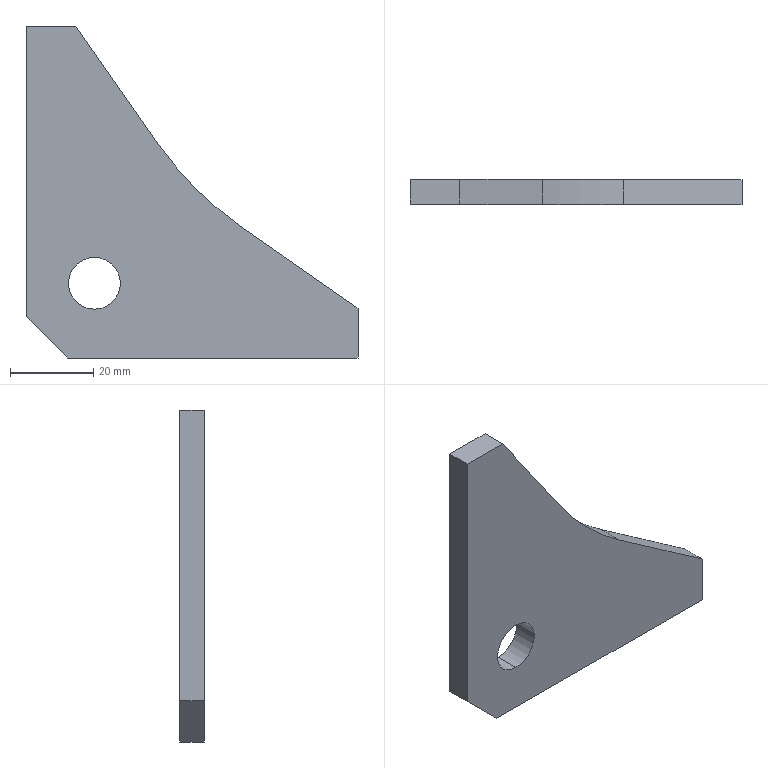Part | SolidWorks | features FlatPattern 1, SMBaseFlange 1, SheetMetal 1 | 1 solid | 12 faces | box 80 x 6 x 80 mm | volume 21113 mm3 | plane 9 | cylinder 3 | commonest cylinder face diameters 12.5 x2 160 x1
STEP:
#1=CARTESIAN_POINT('',(16.5,6.,11.75));
#2=VERTEX_POINT('',#1);
#3=CARTESIAN_POINT('',(16.5,6.,24.25));
#4=VERTEX_POINT('',#3);
#5=CARTESIAN_POINT('',(16.5,6.,18.));
#6=DIRECTION('',(0.,1.,0.));
#7=DIRECTION('',(0.,0.,1.));
#8=AXIS2_PLACEMENT_3D('',#5,#6,#7);
#9=CIRCLE('',#8,6.25);
#10=EDGE_CURVE('',#2,#4,#9,.T.);
#11=ORIENTED_EDGE('',*,*,#10,.T.);
#12=CARTESIAN_POINT('',(16.5,0.,24.25));
#13=VERTEX_POINT('',#12);
#14=CARTESIAN_POINT('',(16.5,6.,24.25));
#15=DIRECTION('',(0.,-1.,0.));
#16=VECTOR('',#15,1000.);
#17=LINE('',#14,#16);
#18=EDGE_CURVE('',#4,#13,#17,.T.);
#19=ORIENTED_EDGE('',*,*,#18,.T.);
#20=CARTESIAN_POINT('',(16.5,0.,11.75));
#21=VERTEX_POINT('',#20);
#22=CARTESIAN_POINT('',(16.5,0.,18.));
#23=DIRECTION('',(0.,1.,0.));
#24=DIRECTION('',(0.,0.,1.));
#25=AXIS2_PLACEMENT_3D('',#22,#23,#24);
#26=CIRCLE('',#25,6.25);
#27=EDGE_CURVE('',#21,#13,#26,.T.);
#28=ORIENTED_EDGE('',*,*,#27,.F.);
#29=CARTESIAN_POINT('',(16.5,6.,11.75));
#30=DIRECTION('',(0.,-1.,0.));
#31=VECTOR('',#30,1000.);
#32=LINE('',#29,#31);
#33=EDGE_CURVE('',#2,#21,#32,.T.);
#34=ORIENTED_EDGE('',*,*,#33,.F.);
#35=EDGE_LOOP('',(#11,#19,#28,#34));
#36=FACE_OUTER_BOUND('',#35,.T.);
#37=CARTESIAN_POINT('',(16.5,6.,18.));
#38=DIRECTION('',(0.,-1.,0.));
#39=DIRECTION('',(0.,0.,-1.));
#40=AXIS2_PLACEMENT_3D('',#37,#38,#39);
#41=CYLINDRICAL_SURFACE('',#40,6.25);
#42=ADVANCED_FACE('',(#36),#41,.F.);
#43=CARTESIAN_POINT('',(80.,6.,12.));
#44=VERTEX_POINT('',#43);
#45=CARTESIAN_POINT('',(80.,6.,0.));
#46=VERTEX_POINT('',#45);
#47=CARTESIAN_POINT('',(80.,6.,12.));
#48=DIRECTION('',(0.,0.,-1.));
#49=VECTOR('',#48,1000.);
#50=LINE('',#47,#49);
#51=EDGE_CURVE('',#44,#46,#50,.T.);
#52=ORIENTED_EDGE('',*,*,#51,.T.);
#53=CARTESIAN_POINT('',(10.,6.,0.));
#54=VERTEX_POINT('',#53);
#55=CARTESIAN_POINT('',(10.,6.,0.));
#56=DIRECTION('',(-1.,0.,0.));
#57=VECTOR('',#56,1000.);
#58=LINE('',#55,#57);
#59=EDGE_CURVE('',#46,#54,#58,.T.);
#60=ORIENTED_EDGE('',*,*,#59,.T.);
#61=CARTESIAN_POINT('',(0.,6.,10.));
#62=VERTEX_POINT('',#61);
#63=CARTESIAN_POINT('',(0.,6.,10.));
#64=DIRECTION('',(-0.7071,0.,0.7071));
#65=VECTOR('',#64,1000.);
#66=LINE('',#63,#65);
#67=EDGE_CURVE('',#54,#62,#66,.T.);
#68=ORIENTED_EDGE('',*,*,#67,.T.);
#69=CARTESIAN_POINT('',(0.,6.,80.));
#70=VERTEX_POINT('',#69);
#71=CARTESIAN_POINT('',(0.,6.,80.));
#72=DIRECTION('',(0.,0.,1.));
#73=VECTOR('',#72,1000.);
#74=LINE('',#71,#73);
#75=EDGE_CURVE('',#62,#70,#74,.T.);
#76=ORIENTED_EDGE('',*,*,#75,.T.);
#77=CARTESIAN_POINT('',(12.,6.,80.));
#78=VERTEX_POINT('',#77);
#79=CARTESIAN_POINT('',(12.,6.,80.));
#80=DIRECTION('',(1.,0.,0.));
#81=VECTOR('',#80,1000.);
#82=LINE('',#79,#81);
#83=EDGE_CURVE('',#70,#78,#82,.T.);
#84=ORIENTED_EDGE('',*,*,#83,.T.);
#85=CARTESIAN_POINT('',(31.904,6.,51.566));
#86=VERTEX_POINT('',#85);
#87=CARTESIAN_POINT('',(31.904,6.,51.566));
#88=DIRECTION('',(0.5735,0.,-0.8192));
#89=VECTOR('',#88,1000.);
#90=LINE('',#87,#89);
#91=EDGE_CURVE('',#78,#86,#90,.T.);
#92=ORIENTED_EDGE('',*,*,#91,.T.);
#93=CARTESIAN_POINT('',(51.566,6.,31.904));
#94=VERTEX_POINT('',#93);
#95=CARTESIAN_POINT('',(97.443,6.,97.443));
#96=DIRECTION('',(0.,-1.,0.));
#97=DIRECTION('',(0.,0.,1.));
#98=AXIS2_PLACEMENT_3D('',#95,#96,#97);
#99=CIRCLE('',#98,80.);
#100=EDGE_CURVE('',#86,#94,#99,.T.);
#101=ORIENTED_EDGE('',*,*,#100,.T.);
#102=CARTESIAN_POINT('',(51.566,6.,31.904));
#103=DIRECTION('',(0.8192,0.,-0.5735));
#104=VECTOR('',#103,1000.);
#105=LINE('',#102,#104);
#106=EDGE_CURVE('',#94,#44,#105,.T.);
#107=ORIENTED_EDGE('',*,*,#106,.T.);
#108=EDGE_LOOP('',(#52,#60,#68,#76,#84,#92,#101,#107));
#109=FACE_OUTER_BOUND('',#108,.T.);
#110=ORIENTED_EDGE('',*,*,#10,.F.);
#111=CARTESIAN_POINT('',(16.5,6.,18.));
#112=DIRECTION('',(0.,1.,0.));
#113=DIRECTION('',(0.,0.,1.));
#114=AXIS2_PLACEMENT_3D('',#111,#112,#113);
#115=CIRCLE('',#114,6.25);
#116=EDGE_CURVE('',#4,#2,#115,.T.);
#117=ORIENTED_EDGE('',*,*,#116,.F.);
#118=EDGE_LOOP('',(#110,#117));
#119=FACE_BOUND('',#118,.T.);
#120=CARTESIAN_POINT('',(97.443,6.,97.443));
#121=DIRECTION('',(0.,1.,0.));
#122=DIRECTION('',(0.,0.,1.));
#123=AXIS2_PLACEMENT_3D('',#120,#121,#122);
#124=PLANE('',#123);
#125=ADVANCED_FACE('',(#109,#119),#124,.T.);
#126=CARTESIAN_POINT('',(80.,0.,12.));
#127=VERTEX_POINT('',#126);
#128=CARTESIAN_POINT('',(80.,0.,0.));
#129=VERTEX_POINT('',#128);
#130=CARTESIAN_POINT('',(80.,0.,12.));
#131=DIRECTION('',(0.,0.,-1.));
#132=VECTOR('',#131,1000.);
#133=LINE('',#130,#132);
#134=EDGE_CURVE('',#127,#129,#133,.T.);
#135=ORIENTED_EDGE('',*,*,#134,.F.);
#136=CARTESIAN_POINT('',(51.566,0.,31.904));
#137=VERTEX_POINT('',#136);
#138=CARTESIAN_POINT('',(51.566,0.,31.904));
#139=DIRECTION('',(0.8192,0.,-0.5735));
#140=VECTOR('',#139,1000.);
#141=LINE('',#138,#140);
#142=EDGE_CURVE('',#137,#127,#141,.T.);
#143=ORIENTED_EDGE('',*,*,#142,.F.);
#144=CARTESIAN_POINT('',(31.904,0.,51.566));
#145=VERTEX_POINT('',#144);
#146=CARTESIAN_POINT('',(97.443,0.,97.443));
#147=DIRECTION('',(0.,-1.,0.));
#148=DIRECTION('',(0.,0.,1.));
#149=AXIS2_PLACEMENT_3D('',#146,#147,#148);
#150=CIRCLE('',#149,80.);
#151=EDGE_CURVE('',#145,#137,#150,.T.);
#152=ORIENTED_EDGE('',*,*,#151,.F.);
#153=CARTESIAN_POINT('',(12.,0.,80.));
#154=VERTEX_POINT('',#153);
#155=CARTESIAN_POINT('',(31.904,0.,51.566));
#156=DIRECTION('',(0.5735,0.,-0.8192));
#157=VECTOR('',#156,1000.);
#158=LINE('',#155,#157);
#159=EDGE_CURVE('',#154,#145,#158,.T.);
#160=ORIENTED_EDGE('',*,*,#159,.F.);
#161=CARTESIAN_POINT('',(0.,0.,80.));
#162=VERTEX_POINT('',#161);
#163=CARTESIAN_POINT('',(12.,0.,80.));
#164=DIRECTION('',(1.,0.,0.));
#165=VECTOR('',#164,1000.);
#166=LINE('',#163,#165);
#167=EDGE_CURVE('',#162,#154,#166,.T.);
#168=ORIENTED_EDGE('',*,*,#167,.F.);
#169=CARTESIAN_POINT('',(0.,0.,10.));
#170=VERTEX_POINT('',#169);
#171=CARTESIAN_POINT('',(0.,0.,80.));
#172=DIRECTION('',(0.,0.,1.));
#173=VECTOR('',#172,1000.);
#174=LINE('',#171,#173);
#175=EDGE_CURVE('',#170,#162,#174,.T.);
#176=ORIENTED_EDGE('',*,*,#175,.F.);
#177=CARTESIAN_POINT('',(10.,0.,0.));
#178=VERTEX_POINT('',#177);
#179=CARTESIAN_POINT('',(0.,0.,10.));
#180=DIRECTION('',(-0.7071,0.,0.7071));
#181=VECTOR('',#180,1000.);
#182=LINE('',#179,#181);
#183=EDGE_CURVE('',#178,#170,#182,.T.);
#184=ORIENTED_EDGE('',*,*,#183,.F.);
#185=CARTESIAN_POINT('',(10.,0.,0.));
#186=DIRECTION('',(-1.,0.,0.));
#187=VECTOR('',#186,1000.);
#188=LINE('',#185,#187);
#189=EDGE_CURVE('',#129,#178,#188,.T.);
#190=ORIENTED_EDGE('',*,*,#189,.F.);
#191=EDGE_LOOP('',(#135,#143,#152,#160,#168,#176,#184,#190));
#192=FACE_OUTER_BOUND('',#191,.T.);
#193=ORIENTED_EDGE('',*,*,#27,.T.);
#194=CARTESIAN_POINT('',(16.5,0.,18.));
#195=DIRECTION('',(0.,1.,0.));
#196=DIRECTION('',(0.,0.,1.));
#197=AXIS2_PLACEMENT_3D('',#194,#195,#196);
#198=CIRCLE('',#197,6.25);
#199=EDGE_CURVE('',#13,#21,#198,.T.);
#200=ORIENTED_EDGE('',*,*,#199,.T.);
#201=EDGE_LOOP('',(#193,#200));
#202=FACE_BOUND('',#201,.T.);
#203=CARTESIAN_POINT('',(97.443,0.,97.443));
#204=DIRECTION('',(0.,1.,0.));
#205=DIRECTION('',(0.,0.,1.));
#206=AXIS2_PLACEMENT_3D('',#203,#204,#205);
#207=PLANE('',#206);
#208=ADVANCED_FACE('',(#192,#202),#207,.F.);
#209=ORIENTED_EDGE('',*,*,#134,.T.);
#210=CARTESIAN_POINT('',(80.,6.,0.));
#211=DIRECTION('',(0.,-1.,0.));
#212=VECTOR('',#211,1000.);
#213=LINE('',#210,#212);
#214=EDGE_CURVE('',#46,#129,#213,.T.);
#215=ORIENTED_EDGE('',*,*,#214,.F.);
#216=ORIENTED_EDGE('',*,*,#51,.F.);
#217=CARTESIAN_POINT('',(80.,6.,12.));
#218=DIRECTION('',(0.,-1.,0.));
#219=VECTOR('',#218,1000.);
#220=LINE('',#217,#219);
#221=EDGE_CURVE('',#44,#127,#220,.T.);
#222=ORIENTED_EDGE('',*,*,#221,.T.);
#223=EDGE_LOOP('',(#209,#215,#216,#222));
#224=FACE_OUTER_BOUND('',#223,.T.);
#225=CARTESIAN_POINT('',(80.,6.,12.));
#226=DIRECTION('',(-1.,0.,0.));
#227=DIRECTION('',(0.,0.,1.));
#228=AXIS2_PLACEMENT_3D('',#225,#226,#227);
#229=PLANE('',#228);
#230=ADVANCED_FACE('',(#224),#229,.F.);
#231=ORIENTED_EDGE('',*,*,#189,.T.);
#232=CARTESIAN_POINT('',(10.,6.,0.));
#233=DIRECTION('',(0.,-1.,0.));
#234=VECTOR('',#233,1000.);
#235=LINE('',#232,#234);
#236=EDGE_CURVE('',#54,#178,#235,.T.);
#237=ORIENTED_EDGE('',*,*,#236,.F.);
#238=ORIENTED_EDGE('',*,*,#59,.F.);
#239=ORIENTED_EDGE('',*,*,#214,.T.);
#240=EDGE_LOOP('',(#231,#237,#238,#239));
#241=FACE_OUTER_BOUND('',#240,.T.);
#242=CARTESIAN_POINT('',(10.,6.,0.));
#243=DIRECTION('',(0.,0.,1.));
#244=DIRECTION('',(1.,0.,0.));
#245=AXIS2_PLACEMENT_3D('',#242,#243,#244);
#246=PLANE('',#245);
#247=ADVANCED_FACE('',(#241),#246,.F.);
#248=ORIENTED_EDGE('',*,*,#183,.T.);
#249=CARTESIAN_POINT('',(0.,6.,10.));
#250=DIRECTION('',(0.,-1.,0.));
#251=VECTOR('',#250,1000.);
#252=LINE('',#249,#251);
#253=EDGE_CURVE('',#62,#170,#252,.T.);
#254=ORIENTED_EDGE('',*,*,#253,.F.);
#255=ORIENTED_EDGE('',*,*,#67,.F.);
#256=ORIENTED_EDGE('',*,*,#236,.T.);
#257=EDGE_LOOP('',(#248,#254,#255,#256));
#258=FACE_OUTER_BOUND('',#257,.T.);
#259=CARTESIAN_POINT('',(0.,6.,10.));
#260=DIRECTION('',(0.7071,0.,0.7071));
#261=DIRECTION('',(0.7071,0.,-0.7071));
#262=AXIS2_PLACEMENT_3D('',#259,#260,#261);
#263=PLANE('',#262);
#264=ADVANCED_FACE('',(#258),#263,.F.);
#265=ORIENTED_EDGE('',*,*,#175,.T.);
#266=CARTESIAN_POINT('',(0.,6.,80.));
#267=DIRECTION('',(0.,-1.,0.));
#268=VECTOR('',#267,1000.);
#269=LINE('',#266,#268);
#270=EDGE_CURVE('',#70,#162,#269,.T.);
#271=ORIENTED_EDGE('',*,*,#270,.F.);
#272=ORIENTED_EDGE('',*,*,#75,.F.);
#273=ORIENTED_EDGE('',*,*,#253,.T.);
#274=EDGE_LOOP('',(#265,#271,#272,#273));
#275=FACE_OUTER_BOUND('',#274,.T.);
#276=CARTESIAN_POINT('',(0.,6.,80.));
#277=DIRECTION('',(1.,0.,0.));
#278=DIRECTION('',(0.,0.,-1.));
#279=AXIS2_PLACEMENT_3D('',#276,#277,#278);
#280=PLANE('',#279);
#281=ADVANCED_FACE('',(#275),#280,.F.);
#282=ORIENTED_EDGE('',*,*,#167,.T.);
#283=CARTESIAN_POINT('',(12.,6.,80.));
#284=DIRECTION('',(0.,-1.,0.));
#285=VECTOR('',#284,1000.);
#286=LINE('',#283,#285);
#287=EDGE_CURVE('',#78,#154,#286,.T.);
#288=ORIENTED_EDGE('',*,*,#287,.F.);
#289=ORIENTED_EDGE('',*,*,#83,.F.);
#290=ORIENTED_EDGE('',*,*,#270,.T.);
#291=EDGE_LOOP('',(#282,#288,#289,#290));
#292=FACE_OUTER_BOUND('',#291,.T.);
#293=CARTESIAN_POINT('',(12.,6.,80.));
#294=DIRECTION('',(0.,0.,-1.));
#295=DIRECTION('',(-1.,0.,0.));
#296=AXIS2_PLACEMENT_3D('',#293,#294,#295);
#297=PLANE('',#296);
#298=ADVANCED_FACE('',(#292),#297,.F.);
#299=ORIENTED_EDGE('',*,*,#159,.T.);
#300=CARTESIAN_POINT('',(31.904,6.,51.566));
#301=DIRECTION('',(0.,-1.,0.));
#302=VECTOR('',#301,1000.);
#303=LINE('',#300,#302);
#304=EDGE_CURVE('',#86,#145,#303,.T.);
#305=ORIENTED_EDGE('',*,*,#304,.F.);
#306=ORIENTED_EDGE('',*,*,#91,.F.);
#307=ORIENTED_EDGE('',*,*,#287,.T.);
#308=EDGE_LOOP('',(#299,#305,#306,#307));
#309=FACE_OUTER_BOUND('',#308,.T.);
#310=CARTESIAN_POINT('',(31.904,6.,51.566));
#311=DIRECTION('',(-0.8192,0.,-0.5735));
#312=DIRECTION('',(-0.5735,0.,0.8192));
#313=AXIS2_PLACEMENT_3D('',#310,#311,#312);
#314=PLANE('',#313);
#315=ADVANCED_FACE('',(#309),#314,.F.);
#316=ORIENTED_EDGE('',*,*,#151,.T.);
#317=CARTESIAN_POINT('',(51.566,6.,31.904));
#318=DIRECTION('',(0.,-1.,0.));
#319=VECTOR('',#318,1000.);
#320=LINE('',#317,#319);
#321=EDGE_CURVE('',#94,#137,#320,.T.);
#322=ORIENTED_EDGE('',*,*,#321,.F.);
#323=ORIENTED_EDGE('',*,*,#100,.F.);
#324=ORIENTED_EDGE('',*,*,#304,.T.);
#325=EDGE_LOOP('',(#316,#322,#323,#324));
#326=FACE_OUTER_BOUND('',#325,.T.);
#327=CARTESIAN_POINT('',(97.443,6.,97.443));
#328=DIRECTION('',(0.,-1.,0.));
#329=DIRECTION('',(0.,0.,-1.));
#330=AXIS2_PLACEMENT_3D('',#327,#328,#329);
#331=CYLINDRICAL_SURFACE('',#330,80.);
#332=ADVANCED_FACE('',(#326),#331,.F.);
#333=ORIENTED_EDGE('',*,*,#142,.T.);
#334=ORIENTED_EDGE('',*,*,#221,.F.);
#335=ORIENTED_EDGE('',*,*,#106,.F.);
#336=ORIENTED_EDGE('',*,*,#321,.T.);
#337=EDGE_LOOP('',(#333,#334,#335,#336));
#338=FACE_OUTER_BOUND('',#337,.T.);
#339=CARTESIAN_POINT('',(51.566,6.,31.904));
#340=DIRECTION('',(-0.5735,0.,-0.8192));
#341=DIRECTION('',(-0.8192,0.,0.5735));
#342=AXIS2_PLACEMENT_3D('',#339,#340,#341);
#343=PLANE('',#342);
#344=ADVANCED_FACE('',(#338),#343,.F.);
#345=ORIENTED_EDGE('',*,*,#18,.F.);
#346=ORIENTED_EDGE('',*,*,#116,.T.);
#347=ORIENTED_EDGE('',*,*,#33,.T.);
#348=ORIENTED_EDGE('',*,*,#199,.F.);
#349=EDGE_LOOP('',(#345,#346,#347,#348));
#350=FACE_OUTER_BOUND('',#349,.T.);
#351=CARTESIAN_POINT('',(16.5,6.,18.));
#352=DIRECTION('',(0.,-1.,0.));
#353=DIRECTION('',(0.,0.,-1.));
#354=AXIS2_PLACEMENT_3D('',#351,#352,#353);
#355=CYLINDRICAL_SURFACE('',#354,6.25);
#356=ADVANCED_FACE('',(#350),#355,.F.);
#357=CLOSED_SHELL('',(#42,#125,#208,#230,#247,#264,#281,#298,#315,#332,#344,#356));
#358=MANIFOLD_SOLID_BREP('',#357);
#359=CARTESIAN_POINT('',(0.,0.,0.));
#360=DIRECTION('',(0.,0.,1.));
#361=DIRECTION('',(1.,0.,0.));
#362=AXIS2_PLACEMENT_3D('',#359,#360,#361);
#363=(LENGTH_UNIT()NAMED_UNIT(*)SI_UNIT(.MILLI.,.METRE.));
#364=UNCERTAINTY_MEASURE_WITH_UNIT(LENGTH_MEASURE(0.00001),#363,'','');
#365=(NAMED_UNIT(*)PLANE_ANGLE_UNIT()SI_UNIT($,.RADIAN.));
#366=(NAMED_UNIT(*)SI_UNIT($,.STERADIAN.)SOLID_ANGLE_UNIT());
#367=(GEOMETRIC_REPRESENTATION_CONTEXT(3)GLOBAL_UNCERTAINTY_ASSIGNED_CONTEXT((#364))GLOBAL_UNIT_ASSIGNED_CONTEXT((#363,#365,#366))REPRESENTATION_CONTEXT('',''));
#368=ADVANCED_BREP_SHAPE_REPRESENTATION('',(#358,#362),#367);